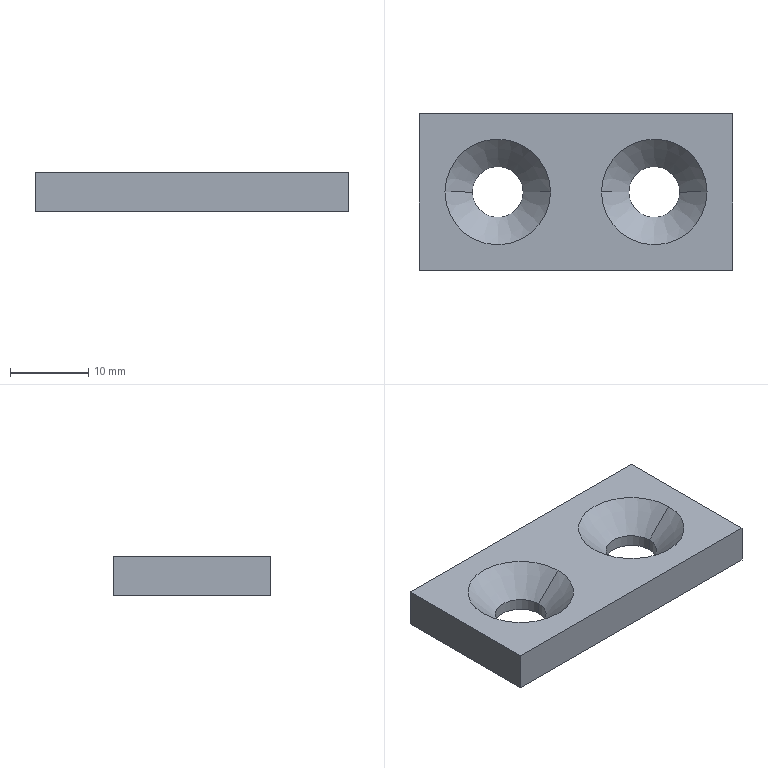Part | STEP file | 0217_012_WSRPM20_40_20 | 1 solid | 14 faces | box 40 x 20 x 5 mm | volume 3328 mm3 | plane 6 | cylinder 4 | cone 4 | commonest cylinder face diameters 6.5 x4
STEP:
#1=CARTESIAN_POINT('',(0.,0.,0.));
#2=DIRECTION('',(0.,0.,1.));
#3=DIRECTION('',(1.,0.,0.));
#4=AXIS2_PLACEMENT_3D('',#1,#2,#3);
#5=CARTESIAN_POINT('',(6.75,10.,1.5));
#6=VERTEX_POINT('',#5);
#7=CARTESIAN_POINT('',(6.75,10.,0.));
#8=VERTEX_POINT('',#7);
#9=CARTESIAN_POINT('',(6.75,10.,0.75));
#10=DIRECTION('',(0.,0.,-1.));
#11=VECTOR('',#10,1.);
#12=LINE('',#9,#11);
#13=CARTESIAN_POINT('',(10.,10.,0.75));
#14=DIRECTION('',(0.,0.,-1.));
#15=DIRECTION('',(-1.,0.,0.));
#16=AXIS2_PLACEMENT_3D('',#13,#14,#15);
#17=CYLINDRICAL_SURFACE('',#16,3.25);
#18=CARTESIAN_POINT('',(6.283,0.));
#19=DIRECTION('',(0.,1.));
#20=VECTOR('',#19,1.);
#21=LINE('',#18,#20);
#22=(GEOMETRIC_REPRESENTATION_CONTEXT(2)PARAMETRIC_REPRESENTATION_CONTEXT()REPRESENTATION_CONTEXT('',''));
#23=DEFINITIONAL_REPRESENTATION('',(#21),#22);
#24=PCURVE('',#17,#23);
#25=CARTESIAN_POINT('',(10.,10.,0.75));
#26=DIRECTION('',(0.,0.,-1.));
#27=DIRECTION('',(-1.,0.,0.));
#28=AXIS2_PLACEMENT_3D('',#25,#26,#27);
#29=CYLINDRICAL_SURFACE('',#28,3.25);
#30=CARTESIAN_POINT('',(0.,0.));
#31=DIRECTION('',(0.,1.));
#32=VECTOR('',#31,1.);
#33=LINE('',#30,#32);
#34=(GEOMETRIC_REPRESENTATION_CONTEXT(2)PARAMETRIC_REPRESENTATION_CONTEXT()REPRESENTATION_CONTEXT('',''));
#35=DEFINITIONAL_REPRESENTATION('',(#33),#34);
#36=PCURVE('',#29,#35);
#37=SURFACE_CURVE('',#12,(#24,#36),.PCURVE_S1.);
#38=EDGE_CURVE('',#6,#8,#37,.T.);
#39=ORIENTED_EDGE('',*,*,#38,.T.);
#40=CARTESIAN_POINT('',(13.25,10.,0.));
#41=VERTEX_POINT('',#40);
#42=CARTESIAN_POINT('',(10.,10.,0.));
#43=DIRECTION('',(0.,0.,-1.));
#44=DIRECTION('',(-1.,0.,0.));
#45=AXIS2_PLACEMENT_3D('',#42,#43,#44);
#46=CIRCLE('',#45,3.25);
#47=CARTESIAN_POINT('',(0.,0.75));
#48=DIRECTION('',(1.,0.));
#49=VECTOR('',#48,1.);
#50=LINE('',#47,#49);
#51=(GEOMETRIC_REPRESENTATION_CONTEXT(2)PARAMETRIC_REPRESENTATION_CONTEXT()REPRESENTATION_CONTEXT('',''));
#52=DEFINITIONAL_REPRESENTATION('',(#50),#51);
#53=PCURVE('',#17,#52);
#54=CARTESIAN_POINT('',(0.,0.,0.));
#55=DIRECTION('',(0.,0.,1.));
#56=DIRECTION('',(1.,0.,0.));
#57=AXIS2_PLACEMENT_3D('',#54,#55,#56);
#58=PLANE('',#57);
#59=CARTESIAN_POINT('',(6.75,10.));
#60=CARTESIAN_POINT('',(6.75,15.629));
#61=CARTESIAN_POINT('',(11.625,12.815));
#62=CARTESIAN_POINT('',(16.5,10.));
#63=CARTESIAN_POINT('',(11.625,7.185));
#64=CARTESIAN_POINT('',(6.75,4.371));
#65=CARTESIAN_POINT('',(6.75,10.));
#66=(BOUNDED_CURVE()B_SPLINE_CURVE(2,(#59,#60,#61,#62,#63,#64,#65),.UNSPECIFIED.,.T.,.F.)B_SPLINE_CURVE_WITH_KNOTS((1,2,2,2,2,1),(-2.094,0.,2.094,4.189,6.283,8.378),.UNSPECIFIED.)CURVE()GEOMETRIC_REPRESENTATION_ITEM()RATIONAL_B_SPLINE_CURVE((1.,0.5,1.,0.5,1.,0.5,1.))REPRESENTATION_ITEM(''));
#67=(GEOMETRIC_REPRESENTATION_CONTEXT(2)PARAMETRIC_REPRESENTATION_CONTEXT()REPRESENTATION_CONTEXT('',''));
#68=DEFINITIONAL_REPRESENTATION('',(#66),#67);
#69=PCURVE('',#58,#68);
#70=SURFACE_CURVE('',#46,(#53,#69),.PCURVE_S1.);
#71=EDGE_CURVE('',#41,#8,#70,.T.);
#72=ORIENTED_EDGE('',*,*,#71,.F.);
#73=CARTESIAN_POINT('',(13.25,10.,1.5));
#74=VERTEX_POINT('',#73);
#75=CARTESIAN_POINT('',(13.25,10.,0.75));
#76=DIRECTION('',(0.,0.,-1.));
#77=VECTOR('',#76,1.);
#78=LINE('',#75,#77);
#79=CARTESIAN_POINT('',(3.142,0.));
#80=DIRECTION('',(0.,1.));
#81=VECTOR('',#80,1.);
#82=LINE('',#79,#81);
#83=(GEOMETRIC_REPRESENTATION_CONTEXT(2)PARAMETRIC_REPRESENTATION_CONTEXT()REPRESENTATION_CONTEXT('',''));
#84=DEFINITIONAL_REPRESENTATION('',(#82),#83);
#85=PCURVE('',#17,#84);
#86=CARTESIAN_POINT('',(3.142,0.));
#87=DIRECTION('',(0.,1.));
#88=VECTOR('',#87,1.);
#89=LINE('',#86,#88);
#90=(GEOMETRIC_REPRESENTATION_CONTEXT(2)PARAMETRIC_REPRESENTATION_CONTEXT()REPRESENTATION_CONTEXT('',''));
#91=DEFINITIONAL_REPRESENTATION('',(#89),#90);
#92=PCURVE('',#29,#91);
#93=SURFACE_CURVE('',#78,(#85,#92),.PCURVE_S1.);
#94=EDGE_CURVE('',#74,#41,#93,.T.);
#95=ORIENTED_EDGE('',*,*,#94,.F.);
#96=CARTESIAN_POINT('',(10.,10.,1.5));
#97=DIRECTION('',(0.,0.,-1.));
#98=DIRECTION('',(-1.,0.,0.));
#99=AXIS2_PLACEMENT_3D('',#96,#97,#98);
#100=CIRCLE('',#99,3.25);
#101=CARTESIAN_POINT('',(0.,-0.75));
#102=DIRECTION('',(1.,0.));
#103=VECTOR('',#102,1.);
#104=LINE('',#101,#103);
#105=(GEOMETRIC_REPRESENTATION_CONTEXT(2)PARAMETRIC_REPRESENTATION_CONTEXT()REPRESENTATION_CONTEXT('',''));
#106=DEFINITIONAL_REPRESENTATION('',(#104),#105);
#107=PCURVE('',#17,#106);
#108=CARTESIAN_POINT('',(10.,10.,5.));
#109=DIRECTION('',(0.,0.,1.));
#110=DIRECTION('',(1.,0.,0.));
#111=AXIS2_PLACEMENT_3D('',#108,#109,#110);
#112=CONICAL_SURFACE('',#111,6.75,0.7854);
#113=CARTESIAN_POINT('',(9.425,-3.5));
#114=DIRECTION('',(-1.,0.));
#115=VECTOR('',#114,1.);
#116=LINE('',#113,#115);
#117=(GEOMETRIC_REPRESENTATION_CONTEXT(2)PARAMETRIC_REPRESENTATION_CONTEXT()REPRESENTATION_CONTEXT('',''));
#118=DEFINITIONAL_REPRESENTATION('',(#116),#117);
#119=PCURVE('',#112,#118);
#120=SURFACE_CURVE('',#100,(#107,#119),.PCURVE_S1.);
#121=EDGE_CURVE('',#74,#6,#120,.T.);
#122=ORIENTED_EDGE('',*,*,#121,.T.);
#123=EDGE_LOOP('',(#39,#72,#95,#122));
#124=FACE_BOUND('',#123,.F.);
#125=ADVANCED_FACE('',(#124),#17,.F.);
#126=CARTESIAN_POINT('',(26.75,10.,1.5));
#127=VERTEX_POINT('',#126);
#128=CARTESIAN_POINT('',(26.75,10.,0.));
#129=VERTEX_POINT('',#128);
#130=CARTESIAN_POINT('',(26.75,10.,0.75));
#131=DIRECTION('',(0.,0.,-1.));
#132=VECTOR('',#131,1.);
#133=LINE('',#130,#132);
#134=CARTESIAN_POINT('',(30.,10.,0.75));
#135=DIRECTION('',(0.,0.,-1.));
#136=DIRECTION('',(-1.,0.,0.));
#137=AXIS2_PLACEMENT_3D('',#134,#135,#136);
#138=CYLINDRICAL_SURFACE('',#137,3.25);
#139=CARTESIAN_POINT('',(6.283,0.));
#140=DIRECTION('',(0.,1.));
#141=VECTOR('',#140,1.);
#142=LINE('',#139,#141);
#143=(GEOMETRIC_REPRESENTATION_CONTEXT(2)PARAMETRIC_REPRESENTATION_CONTEXT()REPRESENTATION_CONTEXT('',''));
#144=DEFINITIONAL_REPRESENTATION('',(#142),#143);
#145=PCURVE('',#138,#144);
#146=CARTESIAN_POINT('',(30.,10.,0.75));
#147=DIRECTION('',(0.,0.,-1.));
#148=DIRECTION('',(-1.,0.,0.));
#149=AXIS2_PLACEMENT_3D('',#146,#147,#148);
#150=CYLINDRICAL_SURFACE('',#149,3.25);
#151=CARTESIAN_POINT('',(0.,0.));
#152=DIRECTION('',(0.,1.));
#153=VECTOR('',#152,1.);
#154=LINE('',#151,#153);
#155=(GEOMETRIC_REPRESENTATION_CONTEXT(2)PARAMETRIC_REPRESENTATION_CONTEXT()REPRESENTATION_CONTEXT('',''));
#156=DEFINITIONAL_REPRESENTATION('',(#154),#155);
#157=PCURVE('',#150,#156);
#158=SURFACE_CURVE('',#133,(#145,#157),.PCURVE_S1.);
#159=EDGE_CURVE('',#127,#129,#158,.T.);
#160=ORIENTED_EDGE('',*,*,#159,.T.);
#161=CARTESIAN_POINT('',(33.25,10.,0.));
#162=VERTEX_POINT('',#161);
#163=CARTESIAN_POINT('',(30.,10.,0.));
#164=DIRECTION('',(0.,0.,-1.));
#165=DIRECTION('',(-1.,0.,0.));
#166=AXIS2_PLACEMENT_3D('',#163,#164,#165);
#167=CIRCLE('',#166,3.25);
#168=CARTESIAN_POINT('',(0.,0.75));
#169=DIRECTION('',(1.,0.));
#170=VECTOR('',#169,1.);
#171=LINE('',#168,#170);
#172=(GEOMETRIC_REPRESENTATION_CONTEXT(2)PARAMETRIC_REPRESENTATION_CONTEXT()REPRESENTATION_CONTEXT('',''));
#173=DEFINITIONAL_REPRESENTATION('',(#171),#172);
#174=PCURVE('',#138,#173);
#175=CARTESIAN_POINT('',(26.75,10.));
#176=CARTESIAN_POINT('',(26.75,15.629));
#177=CARTESIAN_POINT('',(31.625,12.815));
#178=CARTESIAN_POINT('',(36.5,10.));
#179=CARTESIAN_POINT('',(31.625,7.185));
#180=CARTESIAN_POINT('',(26.75,4.371));
#181=CARTESIAN_POINT('',(26.75,10.));
#182=(BOUNDED_CURVE()B_SPLINE_CURVE(2,(#175,#176,#177,#178,#179,#180,#181),.UNSPECIFIED.,.T.,.F.)B_SPLINE_CURVE_WITH_KNOTS((1,2,2,2,2,1),(-2.094,0.,2.094,4.189,6.283,8.378),.UNSPECIFIED.)CURVE()GEOMETRIC_REPRESENTATION_ITEM()RATIONAL_B_SPLINE_CURVE((1.,0.5,1.,0.5,1.,0.5,1.))REPRESENTATION_ITEM(''));
#183=(GEOMETRIC_REPRESENTATION_CONTEXT(2)PARAMETRIC_REPRESENTATION_CONTEXT()REPRESENTATION_CONTEXT('',''));
#184=DEFINITIONAL_REPRESENTATION('',(#182),#183);
#185=PCURVE('',#58,#184);
#186=SURFACE_CURVE('',#167,(#174,#185),.PCURVE_S1.);
#187=EDGE_CURVE('',#162,#129,#186,.T.);
#188=ORIENTED_EDGE('',*,*,#187,.F.);
#189=CARTESIAN_POINT('',(33.25,10.,1.5));
#190=VERTEX_POINT('',#189);
#191=CARTESIAN_POINT('',(33.25,10.,0.75));
#192=DIRECTION('',(0.,0.,-1.));
#193=VECTOR('',#192,1.);
#194=LINE('',#191,#193);
#195=CARTESIAN_POINT('',(3.142,0.));
#196=DIRECTION('',(0.,1.));
#197=VECTOR('',#196,1.);
#198=LINE('',#195,#197);
#199=(GEOMETRIC_REPRESENTATION_CONTEXT(2)PARAMETRIC_REPRESENTATION_CONTEXT()REPRESENTATION_CONTEXT('',''));
#200=DEFINITIONAL_REPRESENTATION('',(#198),#199);
#201=PCURVE('',#138,#200);
#202=CARTESIAN_POINT('',(3.142,0.));
#203=DIRECTION('',(0.,1.));
#204=VECTOR('',#203,1.);
#205=LINE('',#202,#204);
#206=(GEOMETRIC_REPRESENTATION_CONTEXT(2)PARAMETRIC_REPRESENTATION_CONTEXT()REPRESENTATION_CONTEXT('',''));
#207=DEFINITIONAL_REPRESENTATION('',(#205),#206);
#208=PCURVE('',#150,#207);
#209=SURFACE_CURVE('',#194,(#201,#208),.PCURVE_S1.);
#210=EDGE_CURVE('',#190,#162,#209,.T.);
#211=ORIENTED_EDGE('',*,*,#210,.F.);
#212=CARTESIAN_POINT('',(30.,10.,1.5));
#213=DIRECTION('',(0.,0.,-1.));
#214=DIRECTION('',(-1.,0.,0.));
#215=AXIS2_PLACEMENT_3D('',#212,#213,#214);
#216=CIRCLE('',#215,3.25);
#217=CARTESIAN_POINT('',(0.,-0.75));
#218=DIRECTION('',(1.,0.));
#219=VECTOR('',#218,1.);
#220=LINE('',#217,#219);
#221=(GEOMETRIC_REPRESENTATION_CONTEXT(2)PARAMETRIC_REPRESENTATION_CONTEXT()REPRESENTATION_CONTEXT('',''));
#222=DEFINITIONAL_REPRESENTATION('',(#220),#221);
#223=PCURVE('',#138,#222);
#224=CARTESIAN_POINT('',(30.,10.,5.));
#225=DIRECTION('',(0.,0.,1.));
#226=DIRECTION('',(1.,0.,0.));
#227=AXIS2_PLACEMENT_3D('',#224,#225,#226);
#228=CONICAL_SURFACE('',#227,6.75,0.7854);
#229=CARTESIAN_POINT('',(9.425,-3.5));
#230=DIRECTION('',(-1.,0.));
#231=VECTOR('',#230,1.);
#232=LINE('',#229,#231);
#233=(GEOMETRIC_REPRESENTATION_CONTEXT(2)PARAMETRIC_REPRESENTATION_CONTEXT()REPRESENTATION_CONTEXT('',''));
#234=DEFINITIONAL_REPRESENTATION('',(#232),#233);
#235=PCURVE('',#228,#234);
#236=SURFACE_CURVE('',#216,(#223,#235),.PCURVE_S1.);
#237=EDGE_CURVE('',#190,#127,#236,.T.);
#238=ORIENTED_EDGE('',*,*,#237,.T.);
#239=EDGE_LOOP('',(#160,#188,#211,#238));
#240=FACE_BOUND('',#239,.F.);
#241=ADVANCED_FACE('',(#240),#138,.F.);
#242=CARTESIAN_POINT('',(16.75,10.,5.));
#243=VERTEX_POINT('',#242);
#244=CARTESIAN_POINT('',(16.75,10.,5.));
#245=DIRECTION('',(0.7071,0.,0.7071));
#246=VECTOR('',#245,1.);
#247=LINE('',#244,#246);
#248=CARTESIAN_POINT('',(6.283,0.));
#249=DIRECTION('',(0.,1.));
#250=VECTOR('',#249,1.);
#251=LINE('',#248,#250);
#252=(GEOMETRIC_REPRESENTATION_CONTEXT(2)PARAMETRIC_REPRESENTATION_CONTEXT()REPRESENTATION_CONTEXT('',''));
#253=DEFINITIONAL_REPRESENTATION('',(#251),#252);
#254=PCURVE('',#112,#253);
#255=CARTESIAN_POINT('',(10.,10.,5.));
#256=DIRECTION('',(0.,0.,1.));
#257=DIRECTION('',(1.,0.,0.));
#258=AXIS2_PLACEMENT_3D('',#255,#256,#257);
#259=CONICAL_SURFACE('',#258,6.75,0.7854);
#260=CARTESIAN_POINT('',(0.,0.));
#261=DIRECTION('',(0.,1.));
#262=VECTOR('',#261,1.);
#263=LINE('',#260,#262);
#264=(GEOMETRIC_REPRESENTATION_CONTEXT(2)PARAMETRIC_REPRESENTATION_CONTEXT()REPRESENTATION_CONTEXT('',''));
#265=DEFINITIONAL_REPRESENTATION('',(#263),#264);
#266=PCURVE('',#259,#265);
#267=SURFACE_CURVE('',#247,(#254,#266),.PCURVE_S1.);
#268=EDGE_CURVE('',#74,#243,#267,.T.);
#269=ORIENTED_EDGE('',*,*,#268,.T.);
#270=CARTESIAN_POINT('',(3.25,10.,5.));
#271=VERTEX_POINT('',#270);
#272=CARTESIAN_POINT('',(10.,10.,5.));
#273=DIRECTION('',(0.,0.,-1.));
#274=DIRECTION('',(1.,0.,0.));
#275=AXIS2_PLACEMENT_3D('',#272,#273,#274);
#276=CIRCLE('',#275,6.75);
#277=CARTESIAN_POINT('',(6.283,0.));
#278=DIRECTION('',(-1.,0.));
#279=VECTOR('',#278,1.);
#280=LINE('',#277,#279);
#281=(GEOMETRIC_REPRESENTATION_CONTEXT(2)PARAMETRIC_REPRESENTATION_CONTEXT()REPRESENTATION_CONTEXT('',''));
#282=DEFINITIONAL_REPRESENTATION('',(#280),#281);
#283=PCURVE('',#112,#282);
#284=CARTESIAN_POINT('',(0.,0.,5.));
#285=DIRECTION('',(0.,0.,1.));
#286=DIRECTION('',(1.,0.,0.));
#287=AXIS2_PLACEMENT_3D('',#284,#285,#286);
#288=PLANE('',#287);
#289=CARTESIAN_POINT('',(16.75,10.));
#290=CARTESIAN_POINT('',(16.75,-1.691));
#291=CARTESIAN_POINT('',(6.625,4.154));
#292=CARTESIAN_POINT('',(-3.5,10.));
#293=CARTESIAN_POINT('',(6.625,15.846));
#294=CARTESIAN_POINT('',(16.75,21.691));
#295=CARTESIAN_POINT('',(16.75,10.));
#296=(BOUNDED_CURVE()B_SPLINE_CURVE(2,(#289,#290,#291,#292,#293,#294,#295),.UNSPECIFIED.,.T.,.F.)B_SPLINE_CURVE_WITH_KNOTS((1,2,2,2,2,1),(-2.094,0.,2.094,4.189,6.283,8.378),.UNSPECIFIED.)CURVE()GEOMETRIC_REPRESENTATION_ITEM()RATIONAL_B_SPLINE_CURVE((1.,0.5,1.,0.5,1.,0.5,1.))REPRESENTATION_ITEM(''));
#297=(GEOMETRIC_REPRESENTATION_CONTEXT(2)PARAMETRIC_REPRESENTATION_CONTEXT()REPRESENTATION_CONTEXT('',''));
#298=DEFINITIONAL_REPRESENTATION('',(#296),#297);
#299=PCURVE('',#288,#298);
#300=SURFACE_CURVE('',#276,(#283,#299),.PCURVE_S1.);
#301=EDGE_CURVE('',#243,#271,#300,.T.);
#302=ORIENTED_EDGE('',*,*,#301,.T.);
#303=CARTESIAN_POINT('',(3.25,10.,5.));
#304=DIRECTION('',(-0.7071,0.,0.7071));
#305=VECTOR('',#304,1.);
#306=LINE('',#303,#305);
#307=CARTESIAN_POINT('',(3.142,0.));
#308=DIRECTION('',(0.,1.));
#309=VECTOR('',#308,1.);
#310=LINE('',#307,#309);
#311=(GEOMETRIC_REPRESENTATION_CONTEXT(2)PARAMETRIC_REPRESENTATION_CONTEXT()REPRESENTATION_CONTEXT('',''));
#312=DEFINITIONAL_REPRESENTATION('',(#310),#311);
#313=PCURVE('',#112,#312);
#314=CARTESIAN_POINT('',(3.142,0.));
#315=DIRECTION('',(0.,1.));
#316=VECTOR('',#315,1.);
#317=LINE('',#314,#316);
#318=(GEOMETRIC_REPRESENTATION_CONTEXT(2)PARAMETRIC_REPRESENTATION_CONTEXT()REPRESENTATION_CONTEXT('',''));
#319=DEFINITIONAL_REPRESENTATION('',(#317),#318);
#320=PCURVE('',#259,#319);
#321=SURFACE_CURVE('',#306,(#313,#320),.PCURVE_S1.);
#322=EDGE_CURVE('',#6,#271,#321,.T.);
#323=ORIENTED_EDGE('',*,*,#322,.F.);
#324=ORIENTED_EDGE('',*,*,#121,.F.);
#325=EDGE_LOOP('',(#269,#302,#323,#324));
#326=FACE_BOUND('',#325,.F.);
#327=ADVANCED_FACE('',(#326),#112,.F.);
#328=CARTESIAN_POINT('',(36.75,10.,5.));
#329=VERTEX_POINT('',#328);
#330=CARTESIAN_POINT('',(36.75,10.,5.));
#331=DIRECTION('',(0.7071,0.,0.7071));
#332=VECTOR('',#331,1.);
#333=LINE('',#330,#332);
#334=CARTESIAN_POINT('',(6.283,0.));
#335=DIRECTION('',(0.,1.));
#336=VECTOR('',#335,1.);
#337=LINE('',#334,#336);
#338=(GEOMETRIC_REPRESENTATION_CONTEXT(2)PARAMETRIC_REPRESENTATION_CONTEXT()REPRESENTATION_CONTEXT('',''));
#339=DEFINITIONAL_REPRESENTATION('',(#337),#338);
#340=PCURVE('',#228,#339);
#341=CARTESIAN_POINT('',(30.,10.,5.));
#342=DIRECTION('',(0.,0.,1.));
#343=DIRECTION('',(1.,0.,0.));
#344=AXIS2_PLACEMENT_3D('',#341,#342,#343);
#345=CONICAL_SURFACE('',#344,6.75,0.7854);
#346=CARTESIAN_POINT('',(0.,0.));
#347=DIRECTION('',(0.,1.));
#348=VECTOR('',#347,1.);
#349=LINE('',#346,#348);
#350=(GEOMETRIC_REPRESENTATION_CONTEXT(2)PARAMETRIC_REPRESENTATION_CONTEXT()REPRESENTATION_CONTEXT('',''));
#351=DEFINITIONAL_REPRESENTATION('',(#349),#350);
#352=PCURVE('',#345,#351);
#353=SURFACE_CURVE('',#333,(#340,#352),.PCURVE_S1.);
#354=EDGE_CURVE('',#190,#329,#353,.T.);
#355=ORIENTED_EDGE('',*,*,#354,.T.);
#356=CARTESIAN_POINT('',(23.25,10.,5.));
#357=VERTEX_POINT('',#356);
#358=CARTESIAN_POINT('',(30.,10.,5.));
#359=DIRECTION('',(0.,0.,-1.));
#360=DIRECTION('',(1.,0.,0.));
#361=AXIS2_PLACEMENT_3D('',#358,#359,#360);
#362=CIRCLE('',#361,6.75);
#363=CARTESIAN_POINT('',(6.283,0.));
#364=DIRECTION('',(-1.,0.));
#365=VECTOR('',#364,1.);
#366=LINE('',#363,#365);
#367=(GEOMETRIC_REPRESENTATION_CONTEXT(2)PARAMETRIC_REPRESENTATION_CONTEXT()REPRESENTATION_CONTEXT('',''));
#368=DEFINITIONAL_REPRESENTATION('',(#366),#367);
#369=PCURVE('',#228,#368);
#370=CARTESIAN_POINT('',(36.75,10.));
#371=CARTESIAN_POINT('',(36.75,-1.691));
#372=CARTESIAN_POINT('',(26.625,4.154));
#373=CARTESIAN_POINT('',(16.5,10.));
#374=CARTESIAN_POINT('',(26.625,15.846));
#375=CARTESIAN_POINT('',(36.75,21.691));
#376=CARTESIAN_POINT('',(36.75,10.));
#377=(BOUNDED_CURVE()B_SPLINE_CURVE(2,(#370,#371,#372,#373,#374,#375,#376),.UNSPECIFIED.,.T.,.F.)B_SPLINE_CURVE_WITH_KNOTS((1,2,2,2,2,1),(-2.094,0.,2.094,4.189,6.283,8.378),.UNSPECIFIED.)CURVE()GEOMETRIC_REPRESENTATION_ITEM()RATIONAL_B_SPLINE_CURVE((1.,0.5,1.,0.5,1.,0.5,1.))REPRESENTATION_ITEM(''));
#378=(GEOMETRIC_REPRESENTATION_CONTEXT(2)PARAMETRIC_REPRESENTATION_CONTEXT()REPRESENTATION_CONTEXT('',''));
#379=DEFINITIONAL_REPRESENTATION('',(#377),#378);
#380=PCURVE('',#288,#379);
#381=SURFACE_CURVE('',#362,(#369,#380),.PCURVE_S1.);
#382=EDGE_CURVE('',#329,#357,#381,.T.);
#383=ORIENTED_EDGE('',*,*,#382,.T.);
#384=CARTESIAN_POINT('',(23.25,10.,5.));
#385=DIRECTION('',(-0.7071,0.,0.7071));
#386=VECTOR('',#385,1.);
#387=LINE('',#384,#386);
#388=CARTESIAN_POINT('',(3.142,0.));
#389=DIRECTION('',(0.,1.));
#390=VECTOR('',#389,1.);
#391=LINE('',#388,#390);
#392=(GEOMETRIC_REPRESENTATION_CONTEXT(2)PARAMETRIC_REPRESENTATION_CONTEXT()REPRESENTATION_CONTEXT('',''));
#393=DEFINITIONAL_REPRESENTATION('',(#391),#392);
#394=PCURVE('',#228,#393);
#395=CARTESIAN_POINT('',(3.142,0.));
#396=DIRECTION('',(0.,1.));
#397=VECTOR('',#396,1.);
#398=LINE('',#395,#397);
#399=(GEOMETRIC_REPRESENTATION_CONTEXT(2)PARAMETRIC_REPRESENTATION_CONTEXT()REPRESENTATION_CONTEXT('',''));
#400=DEFINITIONAL_REPRESENTATION('',(#398),#399);
#401=PCURVE('',#345,#400);
#402=SURFACE_CURVE('',#387,(#394,#401),.PCURVE_S1.);
#403=EDGE_CURVE('',#127,#357,#402,.T.);
#404=ORIENTED_EDGE('',*,*,#403,.F.);
#405=ORIENTED_EDGE('',*,*,#237,.F.);
#406=EDGE_LOOP('',(#355,#383,#404,#405));
#407=FACE_BOUND('',#406,.F.);
#408=ADVANCED_FACE('',(#407),#228,.F.);
#409=CARTESIAN_POINT('',(0.,20.,0.));
#410=VERTEX_POINT('',#409);
#411=CARTESIAN_POINT('',(0.,0.,0.));
#412=VERTEX_POINT('',#411);
#413=CARTESIAN_POINT('',(0.,0.,0.));
#414=DIRECTION('',(0.,-1.,0.));
#415=VECTOR('',#414,1.);
#416=LINE('',#413,#415);
#417=CARTESIAN_POINT('',(0.,0.));
#418=DIRECTION('',(0.,-1.));
#419=VECTOR('',#418,1.);
#420=LINE('',#417,#419);
#421=(GEOMETRIC_REPRESENTATION_CONTEXT(2)PARAMETRIC_REPRESENTATION_CONTEXT()REPRESENTATION_CONTEXT('',''));
#422=DEFINITIONAL_REPRESENTATION('',(#420),#421);
#423=PCURVE('',#58,#422);
#424=CARTESIAN_POINT('',(0.,0.,0.));
#425=DIRECTION('',(-1.,0.,0.));
#426=DIRECTION('',(0.,0.,1.));
#427=AXIS2_PLACEMENT_3D('',#424,#425,#426);
#428=PLANE('',#427);
#429=CARTESIAN_POINT('',(0.,0.));
#430=DIRECTION('',(0.,-1.));
#431=VECTOR('',#430,1.);
#432=LINE('',#429,#431);
#433=(GEOMETRIC_REPRESENTATION_CONTEXT(2)PARAMETRIC_REPRESENTATION_CONTEXT()REPRESENTATION_CONTEXT('',''));
#434=DEFINITIONAL_REPRESENTATION('',(#432),#433);
#435=PCURVE('',#428,#434);
#436=SURFACE_CURVE('',#416,(#423,#435),.PCURVE_S1.);
#437=EDGE_CURVE('',#410,#412,#436,.T.);
#438=ORIENTED_EDGE('',*,*,#437,.F.);
#439=CARTESIAN_POINT('',(40.,20.,0.));
#440=VERTEX_POINT('',#439);
#441=CARTESIAN_POINT('',(0.,20.,0.));
#442=DIRECTION('',(-1.,0.,0.));
#443=VECTOR('',#442,1.);
#444=LINE('',#441,#443);
#445=CARTESIAN_POINT('',(0.,20.));
#446=DIRECTION('',(-1.,0.));
#447=VECTOR('',#446,1.);
#448=LINE('',#445,#447);
#449=(GEOMETRIC_REPRESENTATION_CONTEXT(2)PARAMETRIC_REPRESENTATION_CONTEXT()REPRESENTATION_CONTEXT('',''));
#450=DEFINITIONAL_REPRESENTATION('',(#448),#449);
#451=PCURVE('',#58,#450);
#452=CARTESIAN_POINT('',(0.,20.,0.));
#453=DIRECTION('',(0.,1.,0.));
#454=DIRECTION('',(0.,0.,1.));
#455=AXIS2_PLACEMENT_3D('',#452,#453,#454);
#456=PLANE('',#455);
#457=CARTESIAN_POINT('',(0.,0.));
#458=DIRECTION('',(0.,-1.));
#459=VECTOR('',#458,1.);
#460=LINE('',#457,#459);
#461=(GEOMETRIC_REPRESENTATION_CONTEXT(2)PARAMETRIC_REPRESENTATION_CONTEXT()REPRESENTATION_CONTEXT('',''));
#462=DEFINITIONAL_REPRESENTATION('',(#460),#461);
#463=PCURVE('',#456,#462);
#464=SURFACE_CURVE('',#444,(#451,#463),.PCURVE_S1.);
#465=EDGE_CURVE('',#440,#410,#464,.T.);
#466=ORIENTED_EDGE('',*,*,#465,.F.);
#467=CARTESIAN_POINT('',(40.,0.,0.));
#468=VERTEX_POINT('',#467);
#469=CARTESIAN_POINT('',(40.,0.,0.));
#470=DIRECTION('',(0.,1.,0.));
#471=VECTOR('',#470,1.);
#472=LINE('',#469,#471);
#473=CARTESIAN_POINT('',(40.,0.));
#474=DIRECTION('',(0.,1.));
#475=VECTOR('',#474,1.);
#476=LINE('',#473,#475);
#477=(GEOMETRIC_REPRESENTATION_CONTEXT(2)PARAMETRIC_REPRESENTATION_CONTEXT()REPRESENTATION_CONTEXT('',''));
#478=DEFINITIONAL_REPRESENTATION('',(#476),#477);
#479=PCURVE('',#58,#478);
#480=CARTESIAN_POINT('',(40.,20.,0.));
#481=DIRECTION('',(1.,0.,0.));
#482=DIRECTION('',(0.,0.,-1.));
#483=AXIS2_PLACEMENT_3D('',#480,#481,#482);
#484=PLANE('',#483);
#485=CARTESIAN_POINT('',(0.,-20.));
#486=DIRECTION('',(0.,1.));
#487=VECTOR('',#486,1.);
#488=LINE('',#485,#487);
#489=(GEOMETRIC_REPRESENTATION_CONTEXT(2)PARAMETRIC_REPRESENTATION_CONTEXT()REPRESENTATION_CONTEXT('',''));
#490=DEFINITIONAL_REPRESENTATION('',(#488),#489);
#491=PCURVE('',#484,#490);
#492=SURFACE_CURVE('',#472,(#479,#491),.PCURVE_S1.);
#493=EDGE_CURVE('',#468,#440,#492,.T.);
#494=ORIENTED_EDGE('',*,*,#493,.F.);
#495=CARTESIAN_POINT('',(0.,0.,0.));
#496=DIRECTION('',(1.,0.,0.));
#497=VECTOR('',#496,1.);
#498=LINE('',#495,#497);
#499=CARTESIAN_POINT('',(0.,0.));
#500=DIRECTION('',(1.,0.));
#501=VECTOR('',#500,1.);
#502=LINE('',#499,#501);
#503=(GEOMETRIC_REPRESENTATION_CONTEXT(2)PARAMETRIC_REPRESENTATION_CONTEXT()REPRESENTATION_CONTEXT('',''));
#504=DEFINITIONAL_REPRESENTATION('',(#502),#503);
#505=PCURVE('',#58,#504);
#506=CARTESIAN_POINT('',(40.,0.,0.));
#507=DIRECTION('',(0.,-1.,0.));
#508=DIRECTION('',(0.,0.,-1.));
#509=AXIS2_PLACEMENT_3D('',#506,#507,#508);
#510=PLANE('',#509);
#511=CARTESIAN_POINT('',(0.,-40.));
#512=DIRECTION('',(0.,1.));
#513=VECTOR('',#512,1.);
#514=LINE('',#511,#513);
#515=(GEOMETRIC_REPRESENTATION_CONTEXT(2)PARAMETRIC_REPRESENTATION_CONTEXT()REPRESENTATION_CONTEXT('',''));
#516=DEFINITIONAL_REPRESENTATION('',(#514),#515);
#517=PCURVE('',#510,#516);
#518=SURFACE_CURVE('',#498,(#505,#517),.PCURVE_S1.);
#519=EDGE_CURVE('',#412,#468,#518,.T.);
#520=ORIENTED_EDGE('',*,*,#519,.F.);
#521=EDGE_LOOP('',(#438,#466,#494,#520));
#522=FACE_BOUND('',#521,.T.);
#523=CARTESIAN_POINT('',(10.,10.,0.));
#524=DIRECTION('',(0.,0.,-1.));
#525=DIRECTION('',(-1.,0.,0.));
#526=AXIS2_PLACEMENT_3D('',#523,#524,#525);
#527=CIRCLE('',#526,3.25);
#528=CARTESIAN_POINT('',(6.75,10.));
#529=CARTESIAN_POINT('',(6.75,15.629));
#530=CARTESIAN_POINT('',(11.625,12.815));
#531=CARTESIAN_POINT('',(16.5,10.));
#532=CARTESIAN_POINT('',(11.625,7.185));
#533=CARTESIAN_POINT('',(6.75,4.371));
#534=CARTESIAN_POINT('',(6.75,10.));
#535=(BOUNDED_CURVE()B_SPLINE_CURVE(2,(#528,#529,#530,#531,#532,#533,#534),.UNSPECIFIED.,.T.,.F.)B_SPLINE_CURVE_WITH_KNOTS((1,2,2,2,2,1),(-2.094,0.,2.094,4.189,6.283,8.378),.UNSPECIFIED.)CURVE()GEOMETRIC_REPRESENTATION_ITEM()RATIONAL_B_SPLINE_CURVE((1.,0.5,1.,0.5,1.,0.5,1.))REPRESENTATION_ITEM(''));
#536=(GEOMETRIC_REPRESENTATION_CONTEXT(2)PARAMETRIC_REPRESENTATION_CONTEXT()REPRESENTATION_CONTEXT('',''));
#537=DEFINITIONAL_REPRESENTATION('',(#535),#536);
#538=PCURVE('',#58,#537);
#539=CARTESIAN_POINT('',(0.,0.75));
#540=DIRECTION('',(1.,0.));
#541=VECTOR('',#540,1.);
#542=LINE('',#539,#541);
#543=(GEOMETRIC_REPRESENTATION_CONTEXT(2)PARAMETRIC_REPRESENTATION_CONTEXT()REPRESENTATION_CONTEXT('',''));
#544=DEFINITIONAL_REPRESENTATION('',(#542),#543);
#545=PCURVE('',#29,#544);
#546=SURFACE_CURVE('',#527,(#538,#545),.PCURVE_S1.);
#547=EDGE_CURVE('',#8,#41,#546,.T.);
#548=ORIENTED_EDGE('',*,*,#547,.F.);
#549=ORIENTED_EDGE('',*,*,#71,.F.);
#550=EDGE_LOOP('',(#548,#549));
#551=FACE_BOUND('',#550,.T.);
#552=CARTESIAN_POINT('',(30.,10.,0.));
#553=DIRECTION('',(0.,0.,-1.));
#554=DIRECTION('',(-1.,0.,0.));
#555=AXIS2_PLACEMENT_3D('',#552,#553,#554);
#556=CIRCLE('',#555,3.25);
#557=CARTESIAN_POINT('',(26.75,10.));
#558=CARTESIAN_POINT('',(26.75,15.629));
#559=CARTESIAN_POINT('',(31.625,12.815));
#560=CARTESIAN_POINT('',(36.5,10.));
#561=CARTESIAN_POINT('',(31.625,7.185));
#562=CARTESIAN_POINT('',(26.75,4.371));
#563=CARTESIAN_POINT('',(26.75,10.));
#564=(BOUNDED_CURVE()B_SPLINE_CURVE(2,(#557,#558,#559,#560,#561,#562,#563),.UNSPECIFIED.,.T.,.F.)B_SPLINE_CURVE_WITH_KNOTS((1,2,2,2,2,1),(-2.094,0.,2.094,4.189,6.283,8.378),.UNSPECIFIED.)CURVE()GEOMETRIC_REPRESENTATION_ITEM()RATIONAL_B_SPLINE_CURVE((1.,0.5,1.,0.5,1.,0.5,1.))REPRESENTATION_ITEM(''));
#565=(GEOMETRIC_REPRESENTATION_CONTEXT(2)PARAMETRIC_REPRESENTATION_CONTEXT()REPRESENTATION_CONTEXT('',''));
#566=DEFINITIONAL_REPRESENTATION('',(#564),#565);
#567=PCURVE('',#58,#566);
#568=CARTESIAN_POINT('',(0.,0.75));
#569=DIRECTION('',(1.,0.));
#570=VECTOR('',#569,1.);
#571=LINE('',#568,#570);
#572=(GEOMETRIC_REPRESENTATION_CONTEXT(2)PARAMETRIC_REPRESENTATION_CONTEXT()REPRESENTATION_CONTEXT('',''));
#573=DEFINITIONAL_REPRESENTATION('',(#571),#572);
#574=PCURVE('',#150,#573);
#575=SURFACE_CURVE('',#556,(#567,#574),.PCURVE_S1.);
#576=EDGE_CURVE('',#129,#162,#575,.T.);
#577=ORIENTED_EDGE('',*,*,#576,.F.);
#578=ORIENTED_EDGE('',*,*,#187,.F.);
#579=EDGE_LOOP('',(#577,#578));
#580=FACE_BOUND('',#579,.T.);
#581=ADVANCED_FACE('',(#522,#551,#580),#58,.F.);
#582=ORIENTED_EDGE('',*,*,#519,.T.);
#583=CARTESIAN_POINT('',(40.,0.,5.));
#584=VERTEX_POINT('',#583);
#585=CARTESIAN_POINT('',(40.,0.,0.));
#586=DIRECTION('',(0.,0.,1.));
#587=VECTOR('',#586,1.);
#588=LINE('',#585,#587);
#589=CARTESIAN_POINT('',(0.,0.));
#590=DIRECTION('',(-1.,0.));
#591=VECTOR('',#590,1.);
#592=LINE('',#589,#591);
#593=(GEOMETRIC_REPRESENTATION_CONTEXT(2)PARAMETRIC_REPRESENTATION_CONTEXT()REPRESENTATION_CONTEXT('',''));
#594=DEFINITIONAL_REPRESENTATION('',(#592),#593);
#595=PCURVE('',#510,#594);
#596=CARTESIAN_POINT('',(0.,-20.));
#597=DIRECTION('',(-1.,0.));
#598=VECTOR('',#597,1.);
#599=LINE('',#596,#598);
#600=(GEOMETRIC_REPRESENTATION_CONTEXT(2)PARAMETRIC_REPRESENTATION_CONTEXT()REPRESENTATION_CONTEXT('',''));
#601=DEFINITIONAL_REPRESENTATION('',(#599),#600);
#602=PCURVE('',#484,#601);
#603=SURFACE_CURVE('',#588,(#595,#602),.PCURVE_S1.);
#604=EDGE_CURVE('',#468,#584,#603,.T.);
#605=ORIENTED_EDGE('',*,*,#604,.T.);
#606=CARTESIAN_POINT('',(0.,0.,5.));
#607=VERTEX_POINT('',#606);
#608=CARTESIAN_POINT('',(40.,0.,5.));
#609=DIRECTION('',(-1.,0.,0.));
#610=VECTOR('',#609,1.);
#611=LINE('',#608,#610);
#612=CARTESIAN_POINT('',(-5.,0.));
#613=DIRECTION('',(0.,-1.));
#614=VECTOR('',#613,1.);
#615=LINE('',#612,#614);
#616=(GEOMETRIC_REPRESENTATION_CONTEXT(2)PARAMETRIC_REPRESENTATION_CONTEXT()REPRESENTATION_CONTEXT('',''));
#617=DEFINITIONAL_REPRESENTATION('',(#615),#616);
#618=PCURVE('',#510,#617);
#619=CARTESIAN_POINT('',(40.,0.));
#620=DIRECTION('',(-1.,0.));
#621=VECTOR('',#620,1.);
#622=LINE('',#619,#621);
#623=(GEOMETRIC_REPRESENTATION_CONTEXT(2)PARAMETRIC_REPRESENTATION_CONTEXT()REPRESENTATION_CONTEXT('',''));
#624=DEFINITIONAL_REPRESENTATION('',(#622),#623);
#625=PCURVE('',#288,#624);
#626=SURFACE_CURVE('',#611,(#618,#625),.PCURVE_S1.);
#627=EDGE_CURVE('',#584,#607,#626,.T.);
#628=ORIENTED_EDGE('',*,*,#627,.T.);
#629=CARTESIAN_POINT('',(0.,0.,0.));
#630=DIRECTION('',(0.,0.,-1.));
#631=VECTOR('',#630,1.);
#632=LINE('',#629,#631);
#633=CARTESIAN_POINT('',(0.,-40.));
#634=DIRECTION('',(1.,0.));
#635=VECTOR('',#634,1.);
#636=LINE('',#633,#635);
#637=(GEOMETRIC_REPRESENTATION_CONTEXT(2)PARAMETRIC_REPRESENTATION_CONTEXT()REPRESENTATION_CONTEXT('',''));
#638=DEFINITIONAL_REPRESENTATION('',(#636),#637);
#639=PCURVE('',#510,#638);
#640=CARTESIAN_POINT('',(0.,0.));
#641=DIRECTION('',(-1.,0.));
#642=VECTOR('',#641,1.);
#643=LINE('',#640,#642);
#644=(GEOMETRIC_REPRESENTATION_CONTEXT(2)PARAMETRIC_REPRESENTATION_CONTEXT()REPRESENTATION_CONTEXT('',''));
#645=DEFINITIONAL_REPRESENTATION('',(#643),#644);
#646=PCURVE('',#428,#645);
#647=SURFACE_CURVE('',#632,(#639,#646),.PCURVE_S1.);
#648=EDGE_CURVE('',#607,#412,#647,.T.);
#649=ORIENTED_EDGE('',*,*,#648,.T.);
#650=EDGE_LOOP('',(#582,#605,#628,#649));
#651=FACE_BOUND('',#650,.T.);
#652=ADVANCED_FACE('',(#651),#510,.T.);
#653=ORIENTED_EDGE('',*,*,#437,.T.);
#654=ORIENTED_EDGE('',*,*,#648,.F.);
#655=CARTESIAN_POINT('',(0.,20.,5.));
#656=VERTEX_POINT('',#655);
#657=CARTESIAN_POINT('',(0.,0.,5.));
#658=DIRECTION('',(0.,1.,0.));
#659=VECTOR('',#658,1.);
#660=LINE('',#657,#659);
#661=CARTESIAN_POINT('',(5.,0.));
#662=DIRECTION('',(0.,1.));
#663=VECTOR('',#662,1.);
#664=LINE('',#661,#663);
#665=(GEOMETRIC_REPRESENTATION_CONTEXT(2)PARAMETRIC_REPRESENTATION_CONTEXT()REPRESENTATION_CONTEXT('',''));
#666=DEFINITIONAL_REPRESENTATION('',(#664),#665);
#667=PCURVE('',#428,#666);
#668=CARTESIAN_POINT('',(0.,0.));
#669=DIRECTION('',(0.,1.));
#670=VECTOR('',#669,1.);
#671=LINE('',#668,#670);
#672=(GEOMETRIC_REPRESENTATION_CONTEXT(2)PARAMETRIC_REPRESENTATION_CONTEXT()REPRESENTATION_CONTEXT('',''));
#673=DEFINITIONAL_REPRESENTATION('',(#671),#672);
#674=PCURVE('',#288,#673);
#675=SURFACE_CURVE('',#660,(#667,#674),.PCURVE_S1.);
#676=EDGE_CURVE('',#607,#656,#675,.T.);
#677=ORIENTED_EDGE('',*,*,#676,.T.);
#678=CARTESIAN_POINT('',(0.,20.,0.));
#679=DIRECTION('',(0.,0.,-1.));
#680=VECTOR('',#679,1.);
#681=LINE('',#678,#680);
#682=CARTESIAN_POINT('',(0.,20.));
#683=DIRECTION('',(-1.,0.));
#684=VECTOR('',#683,1.);
#685=LINE('',#682,#684);
#686=(GEOMETRIC_REPRESENTATION_CONTEXT(2)PARAMETRIC_REPRESENTATION_CONTEXT()REPRESENTATION_CONTEXT('',''));
#687=DEFINITIONAL_REPRESENTATION('',(#685),#686);
#688=PCURVE('',#428,#687);
#689=CARTESIAN_POINT('',(0.,0.));
#690=DIRECTION('',(-1.,0.));
#691=VECTOR('',#690,1.);
#692=LINE('',#689,#691);
#693=(GEOMETRIC_REPRESENTATION_CONTEXT(2)PARAMETRIC_REPRESENTATION_CONTEXT()REPRESENTATION_CONTEXT('',''));
#694=DEFINITIONAL_REPRESENTATION('',(#692),#693);
#695=PCURVE('',#456,#694);
#696=SURFACE_CURVE('',#681,(#688,#695),.PCURVE_S1.);
#697=EDGE_CURVE('',#656,#410,#696,.T.);
#698=ORIENTED_EDGE('',*,*,#697,.T.);
#699=EDGE_LOOP('',(#653,#654,#677,#698));
#700=FACE_BOUND('',#699,.T.);
#701=ADVANCED_FACE('',(#700),#428,.T.);
#702=ORIENTED_EDGE('',*,*,#465,.T.);
#703=ORIENTED_EDGE('',*,*,#697,.F.);
#704=CARTESIAN_POINT('',(40.,20.,5.));
#705=VERTEX_POINT('',#704);
#706=CARTESIAN_POINT('',(0.,20.,5.));
#707=DIRECTION('',(1.,0.,0.));
#708=VECTOR('',#707,1.);
#709=LINE('',#706,#708);
#710=CARTESIAN_POINT('',(5.,0.));
#711=DIRECTION('',(0.,1.));
#712=VECTOR('',#711,1.);
#713=LINE('',#710,#712);
#714=(GEOMETRIC_REPRESENTATION_CONTEXT(2)PARAMETRIC_REPRESENTATION_CONTEXT()REPRESENTATION_CONTEXT('',''));
#715=DEFINITIONAL_REPRESENTATION('',(#713),#714);
#716=PCURVE('',#456,#715);
#717=CARTESIAN_POINT('',(0.,20.));
#718=DIRECTION('',(1.,0.));
#719=VECTOR('',#718,1.);
#720=LINE('',#717,#719);
#721=(GEOMETRIC_REPRESENTATION_CONTEXT(2)PARAMETRIC_REPRESENTATION_CONTEXT()REPRESENTATION_CONTEXT('',''));
#722=DEFINITIONAL_REPRESENTATION('',(#720),#721);
#723=PCURVE('',#288,#722);
#724=SURFACE_CURVE('',#709,(#716,#723),.PCURVE_S1.);
#725=EDGE_CURVE('',#656,#705,#724,.T.);
#726=ORIENTED_EDGE('',*,*,#725,.T.);
#727=CARTESIAN_POINT('',(40.,20.,0.));
#728=DIRECTION('',(0.,0.,-1.));
#729=VECTOR('',#728,1.);
#730=LINE('',#727,#729);
#731=CARTESIAN_POINT('',(0.,40.));
#732=DIRECTION('',(-1.,0.));
#733=VECTOR('',#732,1.);
#734=LINE('',#731,#733);
#735=(GEOMETRIC_REPRESENTATION_CONTEXT(2)PARAMETRIC_REPRESENTATION_CONTEXT()REPRESENTATION_CONTEXT('',''));
#736=DEFINITIONAL_REPRESENTATION('',(#734),#735);
#737=PCURVE('',#456,#736);
#738=CARTESIAN_POINT('',(0.,0.));
#739=DIRECTION('',(1.,0.));
#740=VECTOR('',#739,1.);
#741=LINE('',#738,#740);
#742=(GEOMETRIC_REPRESENTATION_CONTEXT(2)PARAMETRIC_REPRESENTATION_CONTEXT()REPRESENTATION_CONTEXT('',''));
#743=DEFINITIONAL_REPRESENTATION('',(#741),#742);
#744=PCURVE('',#484,#743);
#745=SURFACE_CURVE('',#730,(#737,#744),.PCURVE_S1.);
#746=EDGE_CURVE('',#705,#440,#745,.T.);
#747=ORIENTED_EDGE('',*,*,#746,.T.);
#748=EDGE_LOOP('',(#702,#703,#726,#747));
#749=FACE_BOUND('',#748,.T.);
#750=ADVANCED_FACE('',(#749),#456,.T.);
#751=ORIENTED_EDGE('',*,*,#493,.T.);
#752=ORIENTED_EDGE('',*,*,#746,.F.);
#753=CARTESIAN_POINT('',(40.,20.,5.));
#754=DIRECTION('',(0.,-1.,0.));
#755=VECTOR('',#754,1.);
#756=LINE('',#753,#755);
#757=CARTESIAN_POINT('',(-5.,0.));
#758=DIRECTION('',(0.,-1.));
#759=VECTOR('',#758,1.);
#760=LINE('',#757,#759);
#761=(GEOMETRIC_REPRESENTATION_CONTEXT(2)PARAMETRIC_REPRESENTATION_CONTEXT()REPRESENTATION_CONTEXT('',''));
#762=DEFINITIONAL_REPRESENTATION('',(#760),#761);
#763=PCURVE('',#484,#762);
#764=CARTESIAN_POINT('',(40.,20.));
#765=DIRECTION('',(0.,-1.));
#766=VECTOR('',#765,1.);
#767=LINE('',#764,#766);
#768=(GEOMETRIC_REPRESENTATION_CONTEXT(2)PARAMETRIC_REPRESENTATION_CONTEXT()REPRESENTATION_CONTEXT('',''));
#769=DEFINITIONAL_REPRESENTATION('',(#767),#768);
#770=PCURVE('',#288,#769);
#771=SURFACE_CURVE('',#756,(#763,#770),.PCURVE_S1.);
#772=EDGE_CURVE('',#705,#584,#771,.T.);
#773=ORIENTED_EDGE('',*,*,#772,.T.);
#774=ORIENTED_EDGE('',*,*,#604,.F.);
#775=EDGE_LOOP('',(#751,#752,#773,#774));
#776=FACE_BOUND('',#775,.T.);
#777=ADVANCED_FACE('',(#776),#484,.T.);
#778=ORIENTED_EDGE('',*,*,#547,.F.);
#779=ORIENTED_EDGE('',*,*,#38,.F.);
#780=CARTESIAN_POINT('',(10.,10.,1.5));
#781=DIRECTION('',(0.,0.,-1.));
#782=DIRECTION('',(-1.,0.,0.));
#783=AXIS2_PLACEMENT_3D('',#780,#781,#782);
#784=CIRCLE('',#783,3.25);
#785=CARTESIAN_POINT('',(0.,-0.75));
#786=DIRECTION('',(1.,0.));
#787=VECTOR('',#786,1.);
#788=LINE('',#785,#787);
#789=(GEOMETRIC_REPRESENTATION_CONTEXT(2)PARAMETRIC_REPRESENTATION_CONTEXT()REPRESENTATION_CONTEXT('',''));
#790=DEFINITIONAL_REPRESENTATION('',(#788),#789);
#791=PCURVE('',#29,#790);
#792=CARTESIAN_POINT('',(3.142,-3.5));
#793=DIRECTION('',(-1.,0.));
#794=VECTOR('',#793,1.);
#795=LINE('',#792,#794);
#796=(GEOMETRIC_REPRESENTATION_CONTEXT(2)PARAMETRIC_REPRESENTATION_CONTEXT()REPRESENTATION_CONTEXT('',''));
#797=DEFINITIONAL_REPRESENTATION('',(#795),#796);
#798=PCURVE('',#259,#797);
#799=SURFACE_CURVE('',#784,(#791,#798),.PCURVE_S1.);
#800=EDGE_CURVE('',#6,#74,#799,.T.);
#801=ORIENTED_EDGE('',*,*,#800,.T.);
#802=ORIENTED_EDGE('',*,*,#94,.T.);
#803=EDGE_LOOP('',(#778,#779,#801,#802));
#804=FACE_BOUND('',#803,.F.);
#805=ADVANCED_FACE('',(#804),#29,.F.);
#806=ORIENTED_EDGE('',*,*,#576,.F.);
#807=ORIENTED_EDGE('',*,*,#159,.F.);
#808=CARTESIAN_POINT('',(30.,10.,1.5));
#809=DIRECTION('',(0.,0.,-1.));
#810=DIRECTION('',(-1.,0.,0.));
#811=AXIS2_PLACEMENT_3D('',#808,#809,#810);
#812=CIRCLE('',#811,3.25);
#813=CARTESIAN_POINT('',(0.,-0.75));
#814=DIRECTION('',(1.,0.));
#815=VECTOR('',#814,1.);
#816=LINE('',#813,#815);
#817=(GEOMETRIC_REPRESENTATION_CONTEXT(2)PARAMETRIC_REPRESENTATION_CONTEXT()REPRESENTATION_CONTEXT('',''));
#818=DEFINITIONAL_REPRESENTATION('',(#816),#817);
#819=PCURVE('',#150,#818);
#820=CARTESIAN_POINT('',(3.142,-3.5));
#821=DIRECTION('',(-1.,0.));
#822=VECTOR('',#821,1.);
#823=LINE('',#820,#822);
#824=(GEOMETRIC_REPRESENTATION_CONTEXT(2)PARAMETRIC_REPRESENTATION_CONTEXT()REPRESENTATION_CONTEXT('',''));
#825=DEFINITIONAL_REPRESENTATION('',(#823),#824);
#826=PCURVE('',#345,#825);
#827=SURFACE_CURVE('',#812,(#819,#826),.PCURVE_S1.);
#828=EDGE_CURVE('',#127,#190,#827,.T.);
#829=ORIENTED_EDGE('',*,*,#828,.T.);
#830=ORIENTED_EDGE('',*,*,#210,.T.);
#831=EDGE_LOOP('',(#806,#807,#829,#830));
#832=FACE_BOUND('',#831,.F.);
#833=ADVANCED_FACE('',(#832),#150,.F.);
#834=ORIENTED_EDGE('',*,*,#772,.F.);
#835=ORIENTED_EDGE('',*,*,#725,.F.);
#836=ORIENTED_EDGE('',*,*,#676,.F.);
#837=ORIENTED_EDGE('',*,*,#627,.F.);
#838=EDGE_LOOP('',(#834,#835,#836,#837));
#839=FACE_BOUND('',#838,.T.);
#840=ORIENTED_EDGE('',*,*,#301,.T.);
#841=CARTESIAN_POINT('',(10.,10.,5.));
#842=DIRECTION('',(0.,0.,-1.));
#843=DIRECTION('',(1.,0.,0.));
#844=AXIS2_PLACEMENT_3D('',#841,#842,#843);
#845=CIRCLE('',#844,6.75);
#846=CARTESIAN_POINT('',(16.75,10.));
#847=CARTESIAN_POINT('',(16.75,-1.691));
#848=CARTESIAN_POINT('',(6.625,4.154));
#849=CARTESIAN_POINT('',(-3.5,10.));
#850=CARTESIAN_POINT('',(6.625,15.846));
#851=CARTESIAN_POINT('',(16.75,21.691));
#852=CARTESIAN_POINT('',(16.75,10.));
#853=(BOUNDED_CURVE()B_SPLINE_CURVE(2,(#846,#847,#848,#849,#850,#851,#852),.UNSPECIFIED.,.T.,.F.)B_SPLINE_CURVE_WITH_KNOTS((1,2,2,2,2,1),(-2.094,0.,2.094,4.189,6.283,8.378),.UNSPECIFIED.)CURVE()GEOMETRIC_REPRESENTATION_ITEM()RATIONAL_B_SPLINE_CURVE((1.,0.5,1.,0.5,1.,0.5,1.))REPRESENTATION_ITEM(''));
#854=(GEOMETRIC_REPRESENTATION_CONTEXT(2)PARAMETRIC_REPRESENTATION_CONTEXT()REPRESENTATION_CONTEXT('',''));
#855=DEFINITIONAL_REPRESENTATION('',(#853),#854);
#856=PCURVE('',#288,#855);
#857=CARTESIAN_POINT('',(6.283,0.));
#858=DIRECTION('',(-1.,0.));
#859=VECTOR('',#858,1.);
#860=LINE('',#857,#859);
#861=(GEOMETRIC_REPRESENTATION_CONTEXT(2)PARAMETRIC_REPRESENTATION_CONTEXT()REPRESENTATION_CONTEXT('',''));
#862=DEFINITIONAL_REPRESENTATION('',(#860),#861);
#863=PCURVE('',#259,#862);
#864=SURFACE_CURVE('',#845,(#856,#863),.PCURVE_S1.);
#865=EDGE_CURVE('',#271,#243,#864,.T.);
#866=ORIENTED_EDGE('',*,*,#865,.T.);
#867=EDGE_LOOP('',(#840,#866));
#868=FACE_BOUND('',#867,.T.);
#869=ORIENTED_EDGE('',*,*,#382,.T.);
#870=CARTESIAN_POINT('',(30.,10.,5.));
#871=DIRECTION('',(0.,0.,-1.));
#872=DIRECTION('',(1.,0.,0.));
#873=AXIS2_PLACEMENT_3D('',#870,#871,#872);
#874=CIRCLE('',#873,6.75);
#875=CARTESIAN_POINT('',(36.75,10.));
#876=CARTESIAN_POINT('',(36.75,-1.691));
#877=CARTESIAN_POINT('',(26.625,4.154));
#878=CARTESIAN_POINT('',(16.5,10.));
#879=CARTESIAN_POINT('',(26.625,15.846));
#880=CARTESIAN_POINT('',(36.75,21.691));
#881=CARTESIAN_POINT('',(36.75,10.));
#882=(BOUNDED_CURVE()B_SPLINE_CURVE(2,(#875,#876,#877,#878,#879,#880,#881),.UNSPECIFIED.,.T.,.F.)B_SPLINE_CURVE_WITH_KNOTS((1,2,2,2,2,1),(-2.094,0.,2.094,4.189,6.283,8.378),.UNSPECIFIED.)CURVE()GEOMETRIC_REPRESENTATION_ITEM()RATIONAL_B_SPLINE_CURVE((1.,0.5,1.,0.5,1.,0.5,1.))REPRESENTATION_ITEM(''));
#883=(GEOMETRIC_REPRESENTATION_CONTEXT(2)PARAMETRIC_REPRESENTATION_CONTEXT()REPRESENTATION_CONTEXT('',''));
#884=DEFINITIONAL_REPRESENTATION('',(#882),#883);
#885=PCURVE('',#288,#884);
#886=CARTESIAN_POINT('',(6.283,0.));
#887=DIRECTION('',(-1.,0.));
#888=VECTOR('',#887,1.);
#889=LINE('',#886,#888);
#890=(GEOMETRIC_REPRESENTATION_CONTEXT(2)PARAMETRIC_REPRESENTATION_CONTEXT()REPRESENTATION_CONTEXT('',''));
#891=DEFINITIONAL_REPRESENTATION('',(#889),#890);
#892=PCURVE('',#345,#891);
#893=SURFACE_CURVE('',#874,(#885,#892),.PCURVE_S1.);
#894=EDGE_CURVE('',#357,#329,#893,.T.);
#895=ORIENTED_EDGE('',*,*,#894,.T.);
#896=EDGE_LOOP('',(#869,#895));
#897=FACE_BOUND('',#896,.T.);
#898=ADVANCED_FACE('',(#839,#868,#897),#288,.T.);
#899=ORIENTED_EDGE('',*,*,#865,.T.);
#900=ORIENTED_EDGE('',*,*,#268,.F.);
#901=ORIENTED_EDGE('',*,*,#800,.F.);
#902=ORIENTED_EDGE('',*,*,#322,.T.);
#903=EDGE_LOOP('',(#899,#900,#901,#902));
#904=FACE_BOUND('',#903,.F.);
#905=ADVANCED_FACE('',(#904),#259,.F.);
#906=ORIENTED_EDGE('',*,*,#894,.T.);
#907=ORIENTED_EDGE('',*,*,#354,.F.);
#908=ORIENTED_EDGE('',*,*,#828,.F.);
#909=ORIENTED_EDGE('',*,*,#403,.T.);
#910=EDGE_LOOP('',(#906,#907,#908,#909));
#911=FACE_BOUND('',#910,.F.);
#912=ADVANCED_FACE('',(#911),#345,.F.);
#913=CLOSED_SHELL('',(#125,#241,#327,#408,#581,#652,#701,#750,#777,#805,#833,#898,#905,#912));
#914=MANIFOLD_SOLID_BREP('',#913);
#915=(LENGTH_UNIT()NAMED_UNIT(*)SI_UNIT(.MILLI.,.METRE.));
#916=UNCERTAINTY_MEASURE_WITH_UNIT(LENGTH_MEASURE(0.0000001),#915,'','');
#917=(NAMED_UNIT(*)PLANE_ANGLE_UNIT()SI_UNIT($,.RADIAN.));
#918=(NAMED_UNIT(*)SI_UNIT($,.STERADIAN.)SOLID_ANGLE_UNIT());
#919=(GEOMETRIC_REPRESENTATION_CONTEXT(3)GLOBAL_UNCERTAINTY_ASSIGNED_CONTEXT((#916))GLOBAL_UNIT_ASSIGNED_CONTEXT((#915,#917,#918))REPRESENTATION_CONTEXT('',''));
#920=ADVANCED_BREP_SHAPE_REPRESENTATION('',(#4,#914),#919);